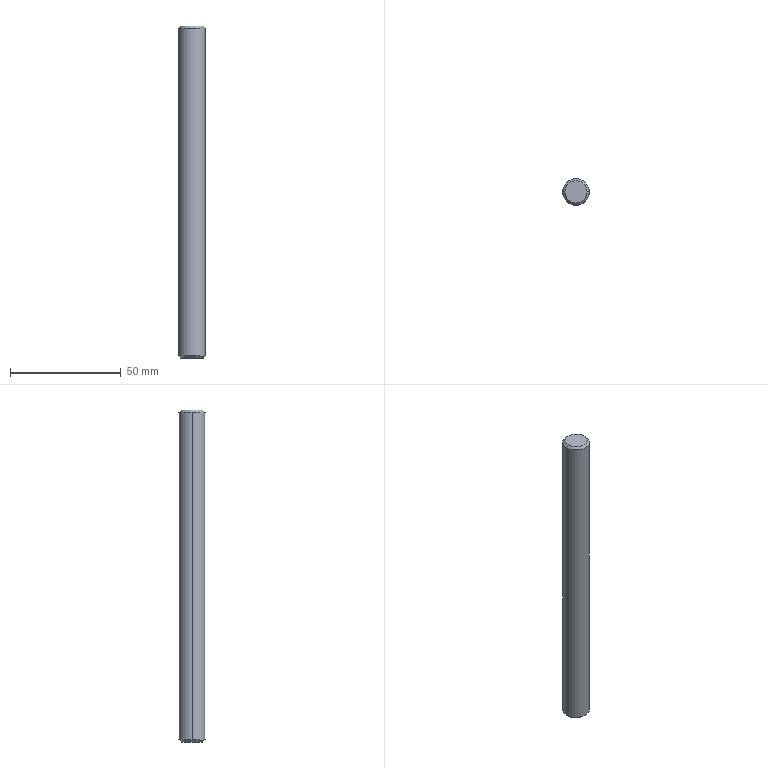Part | STEP file | Guide wheel mechanism revised.sldasm-Part-80 | 1 solid | 12 faces | box 12 x 12 x 150 mm | volume 16178 mm3 | cone 6 | cylinder 4 | plane 2 | commonest cylinder face diameters 6.8 x2 12 x2
STEP:
#1=CARTESIAN_POINT('',(5.,0.,150.));
#2=VERTEX_POINT('',#1);
#3=CARTESIAN_POINT('',(-5.,0.,150.));
#4=VERTEX_POINT('',#3);
#5=CARTESIAN_POINT('',(0.,0.,150.));
#6=DIRECTION('',(0.,0.,1.));
#7=DIRECTION('',(1.,0.,0.));
#8=AXIS2_PLACEMENT_3D('',#5,#6,#7);
#9=CIRCLE('',#8,5.);
#10=EDGE_CURVE('',#2,#4,#9,.T.);
#11=ORIENTED_EDGE('',*,*,#10,.F.);
#12=CARTESIAN_POINT('',(6.,0.,149.));
#13=VERTEX_POINT('',#12);
#14=CARTESIAN_POINT('',(5.,0.,150.));
#15=DIRECTION('',(0.7071,0.,-0.7071));
#16=VECTOR('',#15,1000.);
#17=LINE('',#14,#16);
#18=EDGE_CURVE('',#2,#13,#17,.T.);
#19=ORIENTED_EDGE('',*,*,#18,.T.);
#20=CARTESIAN_POINT('',(-6.,0.,149.));
#21=VERTEX_POINT('',#20);
#22=CARTESIAN_POINT('',(0.,0.,149.));
#23=DIRECTION('',(0.,0.,-1.));
#24=DIRECTION('',(1.,0.,0.));
#25=AXIS2_PLACEMENT_3D('',#22,#23,#24);
#26=CIRCLE('',#25,6.);
#27=EDGE_CURVE('',#21,#13,#26,.T.);
#28=ORIENTED_EDGE('',*,*,#27,.F.);
#29=CARTESIAN_POINT('',(-5.,0.,150.));
#30=DIRECTION('',(-0.7071,0.,-0.7071));
#31=VECTOR('',#30,1000.);
#32=LINE('',#29,#31);
#33=EDGE_CURVE('',#4,#21,#32,.T.);
#34=ORIENTED_EDGE('',*,*,#33,.F.);
#35=EDGE_LOOP('',(#11,#19,#28,#34));
#36=FACE_OUTER_BOUND('',#35,.T.);
#37=CARTESIAN_POINT('',(0.,0.,150.));
#38=DIRECTION('',(0.,0.,-1.));
#39=DIRECTION('',(-1.,0.,0.));
#40=AXIS2_PLACEMENT_3D('',#37,#38,#39);
#41=CONICAL_SURFACE('',#40,5.,0.7854);
#42=ADVANCED_FACE('',(#36),#41,.T.);
#43=CARTESIAN_POINT('',(-5.,0.,0.));
#44=VERTEX_POINT('',#43);
#45=CARTESIAN_POINT('',(5.,0.,0.));
#46=VERTEX_POINT('',#45);
#47=CARTESIAN_POINT('',(0.,0.,0.));
#48=DIRECTION('',(0.,0.,-1.));
#49=DIRECTION('',(1.,0.,0.));
#50=AXIS2_PLACEMENT_3D('',#47,#48,#49);
#51=CIRCLE('',#50,5.);
#52=EDGE_CURVE('',#44,#46,#51,.T.);
#53=ORIENTED_EDGE('',*,*,#52,.F.);
#54=CARTESIAN_POINT('',(-6.,0.,1.));
#55=VERTEX_POINT('',#54);
#56=CARTESIAN_POINT('',(-6.,0.,1.));
#57=DIRECTION('',(-0.7071,0.,0.7071));
#58=VECTOR('',#57,1000.);
#59=LINE('',#56,#58);
#60=EDGE_CURVE('',#44,#55,#59,.T.);
#61=ORIENTED_EDGE('',*,*,#60,.T.);
#62=CARTESIAN_POINT('',(6.,0.,1.));
#63=VERTEX_POINT('',#62);
#64=CARTESIAN_POINT('',(0.,0.,1.));
#65=DIRECTION('',(0.,0.,1.));
#66=DIRECTION('',(1.,0.,0.));
#67=AXIS2_PLACEMENT_3D('',#64,#65,#66);
#68=CIRCLE('',#67,6.);
#69=EDGE_CURVE('',#63,#55,#68,.T.);
#70=ORIENTED_EDGE('',*,*,#69,.F.);
#71=CARTESIAN_POINT('',(6.,0.,1.));
#72=DIRECTION('',(0.7071,0.,0.7071));
#73=VECTOR('',#72,1000.);
#74=LINE('',#71,#73);
#75=EDGE_CURVE('',#46,#63,#74,.T.);
#76=ORIENTED_EDGE('',*,*,#75,.F.);
#77=EDGE_LOOP('',(#53,#61,#70,#76));
#78=FACE_OUTER_BOUND('',#77,.T.);
#79=CARTESIAN_POINT('',(0.,0.,1.));
#80=DIRECTION('',(0.,0.,1.));
#81=DIRECTION('',(1.,0.,0.));
#82=AXIS2_PLACEMENT_3D('',#79,#80,#81);
#83=CONICAL_SURFACE('',#82,6.,0.7854);
#84=ADVANCED_FACE('',(#78),#83,.T.);
#85=CARTESIAN_POINT('',(3.4,0.,20.));
#86=VERTEX_POINT('',#85);
#87=CARTESIAN_POINT('',(-3.4,0.,20.));
#88=VERTEX_POINT('',#87);
#89=CARTESIAN_POINT('',(0.,0.,20.));
#90=DIRECTION('',(0.,0.,-1.));
#91=DIRECTION('',(-1.,0.,0.));
#92=AXIS2_PLACEMENT_3D('',#89,#90,#91);
#93=CIRCLE('',#92,3.4);
#94=EDGE_CURVE('',#86,#88,#93,.T.);
#95=ORIENTED_EDGE('',*,*,#94,.F.);
#96=CARTESIAN_POINT('',(3.4,0.,0.));
#97=VERTEX_POINT('',#96);
#98=CARTESIAN_POINT('',(3.4,0.,0.));
#99=DIRECTION('',(0.,0.,-1.));
#100=VECTOR('',#99,1000.);
#101=LINE('',#98,#100);
#102=EDGE_CURVE('',#86,#97,#101,.T.);
#103=ORIENTED_EDGE('',*,*,#102,.T.);
#104=CARTESIAN_POINT('',(-3.4,0.,0.));
#105=VERTEX_POINT('',#104);
#106=CARTESIAN_POINT('',(0.,0.,0.));
#107=DIRECTION('',(0.,0.,-1.));
#108=DIRECTION('',(-1.,0.,0.));
#109=AXIS2_PLACEMENT_3D('',#106,#107,#108);
#110=CIRCLE('',#109,3.4);
#111=EDGE_CURVE('',#97,#105,#110,.T.);
#112=ORIENTED_EDGE('',*,*,#111,.T.);
#113=CARTESIAN_POINT('',(-3.4,0.,0.));
#114=DIRECTION('',(0.,0.,-1.));
#115=VECTOR('',#114,1000.);
#116=LINE('',#113,#115);
#117=EDGE_CURVE('',#88,#105,#116,.T.);
#118=ORIENTED_EDGE('',*,*,#117,.F.);
#119=EDGE_LOOP('',(#95,#103,#112,#118));
#120=FACE_OUTER_BOUND('',#119,.T.);
#121=CARTESIAN_POINT('',(0.,0.,0.));
#122=DIRECTION('',(0.,0.,-1.));
#123=DIRECTION('',(-1.,0.,0.));
#124=AXIS2_PLACEMENT_3D('',#121,#122,#123);
#125=CYLINDRICAL_SURFACE('',#124,3.4);
#126=ADVANCED_FACE('',(#120),#125,.F.);
#127=CARTESIAN_POINT('',(0.,0.,22.043));
#128=VERTEX_POINT('',#127);
#129=CARTESIAN_POINT('',(-3.4,0.,20.));
#130=DIRECTION('',(-0.8572,0.,-0.515));
#131=VECTOR('',#130,1000.);
#132=LINE('',#129,#131);
#133=EDGE_CURVE('',#128,#88,#132,.T.);
#134=ORIENTED_EDGE('',*,*,#133,.F.);
#135=CARTESIAN_POINT('',(3.4,0.,20.));
#136=DIRECTION('',(0.8572,0.,-0.515));
#137=VECTOR('',#136,1000.);
#138=LINE('',#135,#137);
#139=EDGE_CURVE('',#128,#86,#138,.T.);
#140=ORIENTED_EDGE('',*,*,#139,.T.);
#141=ORIENTED_EDGE('',*,*,#94,.T.);
#142=EDGE_LOOP('',(#134,#140,#141));
#143=FACE_OUTER_BOUND('',#142,.T.);
#144=CARTESIAN_POINT('',(0.,0.,20.));
#145=DIRECTION('',(0.,0.,-1.));
#146=DIRECTION('',(-1.,0.,0.));
#147=AXIS2_PLACEMENT_3D('',#144,#145,#146);
#148=CONICAL_SURFACE('',#147,3.4,1.03);
#149=ADVANCED_FACE('',(#143),#148,.F.);
#150=ORIENTED_EDGE('',*,*,#27,.T.);
#151=CARTESIAN_POINT('',(6.,0.,150.));
#152=DIRECTION('',(0.,0.,-1.));
#153=VECTOR('',#152,1000.);
#154=LINE('',#151,#153);
#155=EDGE_CURVE('',#13,#63,#154,.T.);
#156=ORIENTED_EDGE('',*,*,#155,.T.);
#157=ORIENTED_EDGE('',*,*,#69,.T.);
#158=CARTESIAN_POINT('',(-6.,0.,150.));
#159=DIRECTION('',(0.,0.,-1.));
#160=VECTOR('',#159,1000.);
#161=LINE('',#158,#160);
#162=EDGE_CURVE('',#21,#55,#161,.T.);
#163=ORIENTED_EDGE('',*,*,#162,.F.);
#164=EDGE_LOOP('',(#150,#156,#157,#163));
#165=FACE_OUTER_BOUND('',#164,.T.);
#166=CARTESIAN_POINT('',(0.,0.,150.));
#167=DIRECTION('',(0.,0.,-1.));
#168=DIRECTION('',(-1.,0.,0.));
#169=AXIS2_PLACEMENT_3D('',#166,#167,#168);
#170=CYLINDRICAL_SURFACE('',#169,6.);
#171=ADVANCED_FACE('',(#165),#170,.T.);
#172=ORIENTED_EDGE('',*,*,#155,.F.);
#173=CARTESIAN_POINT('',(0.,0.,149.));
#174=DIRECTION('',(0.,0.,-1.));
#175=DIRECTION('',(1.,0.,0.));
#176=AXIS2_PLACEMENT_3D('',#173,#174,#175);
#177=CIRCLE('',#176,6.);
#178=EDGE_CURVE('',#13,#21,#177,.T.);
#179=ORIENTED_EDGE('',*,*,#178,.T.);
#180=ORIENTED_EDGE('',*,*,#162,.T.);
#181=CARTESIAN_POINT('',(0.,0.,1.));
#182=DIRECTION('',(0.,0.,1.));
#183=DIRECTION('',(1.,0.,0.));
#184=AXIS2_PLACEMENT_3D('',#181,#182,#183);
#185=CIRCLE('',#184,6.);
#186=EDGE_CURVE('',#55,#63,#185,.T.);
#187=ORIENTED_EDGE('',*,*,#186,.T.);
#188=EDGE_LOOP('',(#172,#179,#180,#187));
#189=FACE_OUTER_BOUND('',#188,.T.);
#190=CARTESIAN_POINT('',(0.,0.,150.));
#191=DIRECTION('',(0.,0.,-1.));
#192=DIRECTION('',(-1.,0.,0.));
#193=AXIS2_PLACEMENT_3D('',#190,#191,#192);
#194=CYLINDRICAL_SURFACE('',#193,6.);
#195=ADVANCED_FACE('',(#189),#194,.T.);
#196=CARTESIAN_POINT('',(0.,0.,150.));
#197=DIRECTION('',(0.,0.,1.));
#198=DIRECTION('',(1.,0.,0.));
#199=AXIS2_PLACEMENT_3D('',#196,#197,#198);
#200=CIRCLE('',#199,5.);
#201=EDGE_CURVE('',#4,#2,#200,.T.);
#202=ORIENTED_EDGE('',*,*,#201,.T.);
#203=ORIENTED_EDGE('',*,*,#10,.T.);
#204=EDGE_LOOP('',(#202,#203));
#205=FACE_OUTER_BOUND('',#204,.T.);
#206=CARTESIAN_POINT('',(0.,0.,150.));
#207=DIRECTION('',(0.,0.,1.));
#208=DIRECTION('',(1.,0.,0.));
#209=AXIS2_PLACEMENT_3D('',#206,#207,#208);
#210=PLANE('',#209);
#211=ADVANCED_FACE('',(#205),#210,.T.);
#212=CARTESIAN_POINT('',(0.,0.,0.));
#213=DIRECTION('',(0.,0.,-1.));
#214=DIRECTION('',(1.,0.,0.));
#215=AXIS2_PLACEMENT_3D('',#212,#213,#214);
#216=CIRCLE('',#215,5.);
#217=EDGE_CURVE('',#46,#44,#216,.T.);
#218=ORIENTED_EDGE('',*,*,#217,.T.);
#219=ORIENTED_EDGE('',*,*,#52,.T.);
#220=EDGE_LOOP('',(#218,#219));
#221=FACE_OUTER_BOUND('',#220,.T.);
#222=CARTESIAN_POINT('',(0.,0.,0.));
#223=DIRECTION('',(0.,0.,-1.));
#224=DIRECTION('',(-1.,0.,0.));
#225=AXIS2_PLACEMENT_3D('',#222,#223,#224);
#226=CIRCLE('',#225,3.4);
#227=EDGE_CURVE('',#105,#97,#226,.T.);
#228=ORIENTED_EDGE('',*,*,#227,.F.);
#229=ORIENTED_EDGE('',*,*,#111,.F.);
#230=EDGE_LOOP('',(#228,#229));
#231=FACE_BOUND('',#230,.T.);
#232=CARTESIAN_POINT('',(0.,0.,0.));
#233=DIRECTION('',(0.,0.,1.));
#234=DIRECTION('',(1.,0.,0.));
#235=AXIS2_PLACEMENT_3D('',#232,#233,#234);
#236=PLANE('',#235);
#237=ADVANCED_FACE('',(#221,#231),#236,.F.);
#238=ORIENTED_EDGE('',*,*,#139,.F.);
#239=ORIENTED_EDGE('',*,*,#133,.T.);
#240=CARTESIAN_POINT('',(0.,0.,20.));
#241=DIRECTION('',(0.,0.,-1.));
#242=DIRECTION('',(-1.,0.,0.));
#243=AXIS2_PLACEMENT_3D('',#240,#241,#242);
#244=CIRCLE('',#243,3.4);
#245=EDGE_CURVE('',#88,#86,#244,.T.);
#246=ORIENTED_EDGE('',*,*,#245,.T.);
#247=EDGE_LOOP('',(#238,#239,#246));
#248=FACE_OUTER_BOUND('',#247,.T.);
#249=CARTESIAN_POINT('',(0.,0.,20.));
#250=DIRECTION('',(0.,0.,-1.));
#251=DIRECTION('',(-1.,0.,0.));
#252=AXIS2_PLACEMENT_3D('',#249,#250,#251);
#253=CONICAL_SURFACE('',#252,3.4,1.03);
#254=ADVANCED_FACE('',(#248),#253,.F.);
#255=ORIENTED_EDGE('',*,*,#102,.F.);
#256=ORIENTED_EDGE('',*,*,#245,.F.);
#257=ORIENTED_EDGE('',*,*,#117,.T.);
#258=ORIENTED_EDGE('',*,*,#227,.T.);
#259=EDGE_LOOP('',(#255,#256,#257,#258));
#260=FACE_OUTER_BOUND('',#259,.T.);
#261=CARTESIAN_POINT('',(0.,0.,0.));
#262=DIRECTION('',(0.,0.,-1.));
#263=DIRECTION('',(-1.,0.,0.));
#264=AXIS2_PLACEMENT_3D('',#261,#262,#263);
#265=CYLINDRICAL_SURFACE('',#264,3.4);
#266=ADVANCED_FACE('',(#260),#265,.F.);
#267=ORIENTED_EDGE('',*,*,#60,.F.);
#268=ORIENTED_EDGE('',*,*,#217,.F.);
#269=ORIENTED_EDGE('',*,*,#75,.T.);
#270=ORIENTED_EDGE('',*,*,#186,.F.);
#271=EDGE_LOOP('',(#267,#268,#269,#270));
#272=FACE_OUTER_BOUND('',#271,.T.);
#273=CARTESIAN_POINT('',(0.,0.,1.));
#274=DIRECTION('',(0.,0.,1.));
#275=DIRECTION('',(1.,0.,0.));
#276=AXIS2_PLACEMENT_3D('',#273,#274,#275);
#277=CONICAL_SURFACE('',#276,6.,0.7854);
#278=ADVANCED_FACE('',(#272),#277,.T.);
#279=ORIENTED_EDGE('',*,*,#18,.F.);
#280=ORIENTED_EDGE('',*,*,#201,.F.);
#281=ORIENTED_EDGE('',*,*,#33,.T.);
#282=ORIENTED_EDGE('',*,*,#178,.F.);
#283=EDGE_LOOP('',(#279,#280,#281,#282));
#284=FACE_OUTER_BOUND('',#283,.T.);
#285=CARTESIAN_POINT('',(0.,0.,150.));
#286=DIRECTION('',(0.,0.,-1.));
#287=DIRECTION('',(-1.,0.,0.));
#288=AXIS2_PLACEMENT_3D('',#285,#286,#287);
#289=CONICAL_SURFACE('',#288,5.,0.7854);
#290=ADVANCED_FACE('',(#284),#289,.T.);
#291=CLOSED_SHELL('',(#42,#84,#126,#149,#171,#195,#211,#237,#254,#266,#278,#290));
#292=MANIFOLD_SOLID_BREP('',#291);
#293=CARTESIAN_POINT('',(0.,0.,0.));
#294=DIRECTION('',(0.,0.,1.));
#295=DIRECTION('',(1.,0.,0.));
#296=AXIS2_PLACEMENT_3D('',#293,#294,#295);
#297=(LENGTH_UNIT()NAMED_UNIT(*)SI_UNIT(.MILLI.,.METRE.));
#298=UNCERTAINTY_MEASURE_WITH_UNIT(LENGTH_MEASURE(0.00001),#297,'','');
#299=(NAMED_UNIT(*)PLANE_ANGLE_UNIT()SI_UNIT($,.RADIAN.));
#300=(NAMED_UNIT(*)SI_UNIT($,.STERADIAN.)SOLID_ANGLE_UNIT());
#301=(GEOMETRIC_REPRESENTATION_CONTEXT(3)GLOBAL_UNCERTAINTY_ASSIGNED_CONTEXT((#298))GLOBAL_UNIT_ASSIGNED_CONTEXT((#297,#299,#300))REPRESENTATION_CONTEXT('',''));
#302=ADVANCED_BREP_SHAPE_REPRESENTATION('',(#292,#296),#301);